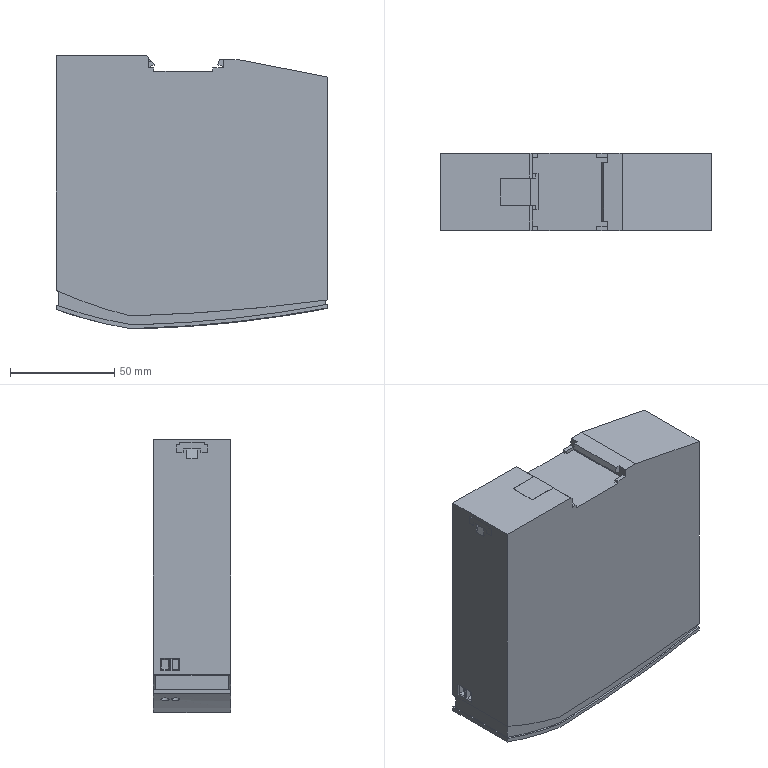Part | SolidWorks | features BaseBody 1 | 1 solid | 192 faces | box 130 x 37 x 131 mm | volume 590430 mm3 | plane 159 | cylinder 33 | commonest cylinder face diameters 4 x14 396.105 x3 399.895 x3 1800 x3 3 x2 400 x2